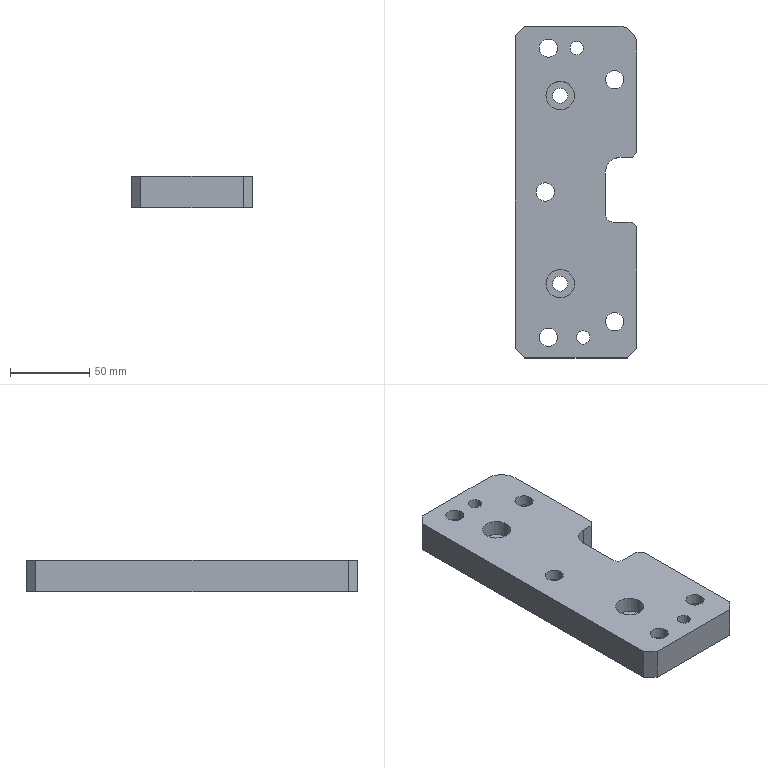Part | STEP file | lll_id3610_x_t | 1 solid | 41 faces | box 77 x 210 x 20 mm | volume 276670 mm3 | plane 22 | cylinder 19 | commonest cylinder face diameters 11.509 x5 18.007 x5 8.505 x2 9.55 x2 18 x2 10 x1
STEP:
#1=CARTESIAN_POINT('',(3739.,91.5,2.5));
#2=VERTEX_POINT('',#1);
#3=CARTESIAN_POINT('',(3739.,23.5,2.5));
#4=VERTEX_POINT('',#3);
#5=CARTESIAN_POINT('',(3739.,-58.5,2.5));
#6=DIRECTION('',(0.,-1.,0.));
#7=VECTOR('',#6,1.);
#8=LINE('',#5,#7);
#9=EDGE_CURVE('',#2,#4,#8,.T.);
#10=ORIENTED_EDGE('',*,*,#9,.F.);
#11=CARTESIAN_POINT('',(3739.,91.5,22.5));
#12=VERTEX_POINT('',#11);
#13=CARTESIAN_POINT('',(3739.,91.5,-81.5));
#14=DIRECTION('',(0.,0.,1.));
#15=VECTOR('',#14,1.);
#16=LINE('',#13,#15);
#17=EDGE_CURVE('',#2,#12,#16,.T.);
#18=ORIENTED_EDGE('',*,*,#17,.T.);
#19=CARTESIAN_POINT('',(3739.,23.5,22.5));
#20=VERTEX_POINT('',#19);
#21=CARTESIAN_POINT('',(3739.,-58.5,22.5));
#22=DIRECTION('',(0.,1.,0.));
#23=VECTOR('',#22,1.);
#24=LINE('',#21,#23);
#25=EDGE_CURVE('',#20,#12,#24,.T.);
#26=ORIENTED_EDGE('',*,*,#25,.F.);
#27=CARTESIAN_POINT('',(3739.,23.5,-81.5));
#28=DIRECTION('',(0.,0.,-1.));
#29=VECTOR('',#28,1.);
#30=LINE('',#27,#29);
#31=EDGE_CURVE('',#20,#4,#30,.T.);
#32=ORIENTED_EDGE('',*,*,#31,.T.);
#33=EDGE_LOOP('',(#10,#18,#26,#32));
#34=FACE_OUTER_BOUND('',#33,.T.);
#35=CARTESIAN_POINT('',(3739.,-58.5,-81.5));
#36=DIRECTION('',(1.,0.,0.));
#37=DIRECTION('',(0.,0.,-1.));
#38=AXIS2_PLACEMENT_3D('',#35,#36,#37);
#39=PLANE('',#38);
#40=ADVANCED_FACE('',(#34),#39,.T.);
#41=CARTESIAN_POINT('',(3690.004,-1.5,2.5));
#42=VERTEX_POINT('',#41);
#43=CARTESIAN_POINT('',(3681.,-1.5,2.5));
#44=DIRECTION('',(0.,0.,1.));
#45=DIRECTION('',(1.,0.,0.));
#46=AXIS2_PLACEMENT_3D('',#43,#44,#45);
#47=CIRCLE('',#46,9.004);
#48=EDGE_CURVE('',#42,#42,#47,.T.);
#49=ORIENTED_EDGE('',*,*,#48,.T.);
#50=EDGE_LOOP('',(#49));
#51=FACE_BOUND('',#50,.T.);
#52=CARTESIAN_POINT('',(3692.004,89.5,2.5));
#53=VERTEX_POINT('',#52);
#54=CARTESIAN_POINT('',(3683.,89.5,2.5));
#55=DIRECTION('',(0.,0.,1.));
#56=DIRECTION('',(1.,0.,0.));
#57=AXIS2_PLACEMENT_3D('',#54,#55,#56);
#58=CIRCLE('',#57,9.004);
#59=EDGE_CURVE('',#53,#53,#58,.T.);
#60=ORIENTED_EDGE('',*,*,#59,.T.);
#61=EDGE_LOOP('',(#60));
#62=FACE_BOUND('',#61,.T.);
#63=CARTESIAN_POINT('',(3705.253,89.5,2.5));
#64=VERTEX_POINT('',#63);
#65=CARTESIAN_POINT('',(3701.,89.5,2.5));
#66=DIRECTION('',(0.,0.,-1.));
#67=DIRECTION('',(1.,0.,0.));
#68=AXIS2_PLACEMENT_3D('',#65,#66,#67);
#69=CIRCLE('',#68,4.253);
#70=EDGE_CURVE('',#64,#64,#69,.T.);
#71=ORIENTED_EDGE('',*,*,#70,.F.);
#72=EDGE_LOOP('',(#71));
#73=FACE_BOUND('',#72,.T.);
#74=CARTESIAN_POINT('',(3692.004,-93.5,2.5));
#75=VERTEX_POINT('',#74);
#76=CARTESIAN_POINT('',(3683.,-93.5,2.5));
#77=DIRECTION('',(0.,0.,1.));
#78=DIRECTION('',(1.,0.,0.));
#79=AXIS2_PLACEMENT_3D('',#76,#77,#78);
#80=CIRCLE('',#79,9.004);
#81=EDGE_CURVE('',#75,#75,#80,.T.);
#82=ORIENTED_EDGE('',*,*,#81,.T.);
#83=EDGE_LOOP('',(#82));
#84=FACE_BOUND('',#83,.T.);
#85=CARTESIAN_POINT('',(3709.253,-93.5,2.5));
#86=VERTEX_POINT('',#85);
#87=CARTESIAN_POINT('',(3705.,-93.5,2.5));
#88=DIRECTION('',(0.,0.,-1.));
#89=DIRECTION('',(1.,0.,0.));
#90=AXIS2_PLACEMENT_3D('',#87,#88,#89);
#91=CIRCLE('',#90,4.253);
#92=EDGE_CURVE('',#86,#86,#91,.T.);
#93=ORIENTED_EDGE('',*,*,#92,.F.);
#94=EDGE_LOOP('',(#93));
#95=FACE_BOUND('',#94,.T.);
#96=CARTESIAN_POINT('',(3685.725,-59.5,2.5));
#97=VERTEX_POINT('',#96);
#98=CARTESIAN_POINT('',(3690.5,-59.5,2.5));
#99=DIRECTION('',(0.,0.,-1.));
#100=DIRECTION('',(-1.,0.,0.));
#101=AXIS2_PLACEMENT_3D('',#98,#99,#100);
#102=CIRCLE('',#101,4.775);
#103=EDGE_CURVE('',#97,#97,#102,.T.);
#104=ORIENTED_EDGE('',*,*,#103,.F.);
#105=EDGE_LOOP('',(#104));
#106=FACE_BOUND('',#105,.T.);
#107=CARTESIAN_POINT('',(3685.725,59.5,2.5));
#108=VERTEX_POINT('',#107);
#109=CARTESIAN_POINT('',(3690.5,59.5,2.5));
#110=DIRECTION('',(0.,0.,-1.));
#111=DIRECTION('',(-1.,0.,0.));
#112=AXIS2_PLACEMENT_3D('',#109,#110,#111);
#113=CIRCLE('',#112,4.775);
#114=EDGE_CURVE('',#108,#108,#113,.T.);
#115=ORIENTED_EDGE('',*,*,#114,.F.);
#116=EDGE_LOOP('',(#115));
#117=FACE_BOUND('',#116,.T.);
#118=CARTESIAN_POINT('',(3734.004,-83.5,2.5));
#119=VERTEX_POINT('',#118);
#120=CARTESIAN_POINT('',(3725.,-83.5,2.5));
#121=DIRECTION('',(0.,0.,1.));
#122=DIRECTION('',(1.,0.,0.));
#123=AXIS2_PLACEMENT_3D('',#120,#121,#122);
#124=CIRCLE('',#123,9.004);
#125=EDGE_CURVE('',#119,#119,#124,.T.);
#126=ORIENTED_EDGE('',*,*,#125,.T.);
#127=EDGE_LOOP('',(#126));
#128=FACE_BOUND('',#127,.T.);
#129=CARTESIAN_POINT('',(3734.004,69.5,2.5));
#130=VERTEX_POINT('',#129);
#131=CARTESIAN_POINT('',(3725.,69.5,2.5));
#132=DIRECTION('',(0.,0.,1.));
#133=DIRECTION('',(1.,0.,0.));
#134=AXIS2_PLACEMENT_3D('',#131,#132,#133);
#135=CIRCLE('',#134,9.004);
#136=EDGE_CURVE('',#130,#130,#135,.T.);
#137=ORIENTED_EDGE('',*,*,#136,.T.);
#138=EDGE_LOOP('',(#137));
#139=FACE_BOUND('',#138,.T.);
#140=CARTESIAN_POINT('',(3668.,103.5,2.5));
#141=VERTEX_POINT('',#140);
#142=CARTESIAN_POINT('',(3727.,103.5,2.5));
#143=VERTEX_POINT('',#142);
#144=CARTESIAN_POINT('',(3692.5,103.5,2.5));
#145=DIRECTION('',(1.,0.,0.));
#146=VECTOR('',#145,1.);
#147=LINE('',#144,#146);
#148=EDGE_CURVE('',#141,#143,#147,.T.);
#149=ORIENTED_EDGE('',*,*,#148,.T.);
#150=CARTESIAN_POINT('',(3727.,91.5,2.5));
#151=DIRECTION('',(0.,0.,-1.));
#152=DIRECTION('',(1.,0.,0.));
#153=AXIS2_PLACEMENT_3D('',#150,#151,#152);
#154=CIRCLE('',#153,12.);
#155=EDGE_CURVE('',#143,#2,#154,.T.);
#156=ORIENTED_EDGE('',*,*,#155,.T.);
#157=ORIENTED_EDGE('',*,*,#9,.T.);
#158=CARTESIAN_POINT('',(3736.,20.5,2.5));
#159=VERTEX_POINT('',#158);
#160=CARTESIAN_POINT('',(3814.88,99.38,2.5));
#161=DIRECTION('',(-0.7071,-0.7071,0.));
#162=VECTOR('',#161,1.);
#163=LINE('',#160,#162);
#164=EDGE_CURVE('',#4,#159,#163,.T.);
#165=ORIENTED_EDGE('',*,*,#164,.T.);
#166=CARTESIAN_POINT('',(3729.,20.5,2.5));
#167=VERTEX_POINT('',#166);
#168=CARTESIAN_POINT('',(4001.917,20.5,2.5));
#169=DIRECTION('',(-1.,0.,0.));
#170=VECTOR('',#169,1.);
#171=LINE('',#168,#170);
#172=EDGE_CURVE('',#159,#167,#171,.T.);
#173=ORIENTED_EDGE('',*,*,#172,.T.);
#174=CARTESIAN_POINT('',(3719.,10.5,2.5));
#175=VERTEX_POINT('',#174);
#176=CARTESIAN_POINT('',(3729.,10.5,2.5));
#177=DIRECTION('',(0.,0.,1.));
#178=DIRECTION('',(1.,0.,0.));
#179=AXIS2_PLACEMENT_3D('',#176,#177,#178);
#180=CIRCLE('',#179,10.);
#181=EDGE_CURVE('',#167,#175,#180,.T.);
#182=ORIENTED_EDGE('',*,*,#181,.T.);
#183=CARTESIAN_POINT('',(3719.,-15.5,2.5));
#184=VERTEX_POINT('',#183);
#185=CARTESIAN_POINT('',(3719.,-87.658,2.5));
#186=DIRECTION('',(0.,-1.,0.));
#187=VECTOR('',#186,1.);
#188=LINE('',#185,#187);
#189=EDGE_CURVE('',#175,#184,#188,.T.);
#190=ORIENTED_EDGE('',*,*,#189,.T.);
#191=CARTESIAN_POINT('',(3724.,-20.5,2.5));
#192=VERTEX_POINT('',#191);
#193=CARTESIAN_POINT('',(3724.,-15.5,2.5));
#194=DIRECTION('',(0.,0.,1.));
#195=DIRECTION('',(1.,0.,0.));
#196=AXIS2_PLACEMENT_3D('',#193,#194,#195);
#197=CIRCLE('',#196,5.);
#198=EDGE_CURVE('',#184,#192,#197,.T.);
#199=ORIENTED_EDGE('',*,*,#198,.T.);
#200=CARTESIAN_POINT('',(3736.,-20.5,2.5));
#201=VERTEX_POINT('',#200);
#202=CARTESIAN_POINT('',(4001.917,-20.5,2.5));
#203=DIRECTION('',(1.,0.,0.));
#204=VECTOR('',#203,1.);
#205=LINE('',#202,#204);
#206=EDGE_CURVE('',#192,#201,#205,.T.);
#207=ORIENTED_EDGE('',*,*,#206,.T.);
#208=CARTESIAN_POINT('',(3739.,-23.5,2.5));
#209=VERTEX_POINT('',#208);
#210=CARTESIAN_POINT('',(3902.537,-187.037,2.5));
#211=DIRECTION('',(0.7071,-0.7071,0.));
#212=VECTOR('',#211,1.);
#213=LINE('',#210,#212);
#214=EDGE_CURVE('',#201,#209,#213,.T.);
#215=ORIENTED_EDGE('',*,*,#214,.T.);
#216=CARTESIAN_POINT('',(3739.,-100.5,2.5));
#217=VERTEX_POINT('',#216);
#218=CARTESIAN_POINT('',(3739.,-58.5,2.5));
#219=DIRECTION('',(0.,-1.,0.));
#220=VECTOR('',#219,1.);
#221=LINE('',#218,#220);
#222=EDGE_CURVE('',#209,#217,#221,.T.);
#223=ORIENTED_EDGE('',*,*,#222,.T.);
#224=CARTESIAN_POINT('',(3733.,-106.5,2.5));
#225=VERTEX_POINT('',#224);
#226=CARTESIAN_POINT('',(3733.,-106.5,2.5));
#227=DIRECTION('',(-0.7071,-0.7071,0.));
#228=VECTOR('',#227,1.);
#229=LINE('',#226,#228);
#230=EDGE_CURVE('',#217,#225,#229,.T.);
#231=ORIENTED_EDGE('',*,*,#230,.T.);
#232=CARTESIAN_POINT('',(3668.,-106.5,2.5));
#233=VERTEX_POINT('',#232);
#234=CARTESIAN_POINT('',(3692.5,-106.5,2.5));
#235=DIRECTION('',(-1.,0.,0.));
#236=VECTOR('',#235,1.);
#237=LINE('',#234,#236);
#238=EDGE_CURVE('',#225,#233,#237,.T.);
#239=ORIENTED_EDGE('',*,*,#238,.T.);
#240=CARTESIAN_POINT('',(3662.,-100.5,2.5));
#241=VERTEX_POINT('',#240);
#242=CARTESIAN_POINT('',(3662.,-100.5,2.5));
#243=DIRECTION('',(-0.7071,0.7071,0.));
#244=VECTOR('',#243,1.);
#245=LINE('',#242,#244);
#246=EDGE_CURVE('',#233,#241,#245,.T.);
#247=ORIENTED_EDGE('',*,*,#246,.T.);
#248=CARTESIAN_POINT('',(3662.,97.5,2.5));
#249=VERTEX_POINT('',#248);
#250=CARTESIAN_POINT('',(3662.,-87.658,2.5));
#251=DIRECTION('',(0.,-1.,0.));
#252=VECTOR('',#251,1.);
#253=LINE('',#250,#252);
#254=EDGE_CURVE('',#249,#241,#253,.T.);
#255=ORIENTED_EDGE('',*,*,#254,.F.);
#256=CARTESIAN_POINT('',(3662.,97.5,2.5));
#257=DIRECTION('',(0.7071,0.7071,0.));
#258=VECTOR('',#257,1.);
#259=LINE('',#256,#258);
#260=EDGE_CURVE('',#249,#141,#259,.T.);
#261=ORIENTED_EDGE('',*,*,#260,.T.);
#262=EDGE_LOOP('',(#149,#156,#157,#165,#173,#182,#190,#199,#207,#215,#223,#231,#239,#247,#255,#261));
#263=FACE_BOUND('',#262,.T.);
#264=CARTESIAN_POINT('',(4001.917,-87.658,2.5));
#265=DIRECTION('',(0.,0.,1.));
#266=DIRECTION('',(0.,-1.,0.));
#267=AXIS2_PLACEMENT_3D('',#264,#265,#266);
#268=PLANE('',#267);
#269=ADVANCED_FACE('',(#51,#62,#73,#84,#95,#106,#117,#128,#139,#263),#268,.F.);
#270=CARTESIAN_POINT('',(3739.,-100.5,22.5));
#271=VERTEX_POINT('',#270);
#272=CARTESIAN_POINT('',(3739.,-23.5,22.5));
#273=VERTEX_POINT('',#272);
#274=CARTESIAN_POINT('',(3739.,-58.5,22.5));
#275=DIRECTION('',(0.,1.,0.));
#276=VECTOR('',#275,1.);
#277=LINE('',#274,#276);
#278=EDGE_CURVE('',#271,#273,#277,.T.);
#279=ORIENTED_EDGE('',*,*,#278,.F.);
#280=CARTESIAN_POINT('',(3739.,-100.5,-81.5));
#281=DIRECTION('',(0.,0.,-1.));
#282=VECTOR('',#281,1.);
#283=LINE('',#280,#282);
#284=EDGE_CURVE('',#271,#217,#283,.T.);
#285=ORIENTED_EDGE('',*,*,#284,.T.);
#286=ORIENTED_EDGE('',*,*,#222,.F.);
#287=CARTESIAN_POINT('',(3739.,-23.5,-81.5));
#288=DIRECTION('',(0.,0.,1.));
#289=VECTOR('',#288,1.);
#290=LINE('',#287,#289);
#291=EDGE_CURVE('',#209,#273,#290,.T.);
#292=ORIENTED_EDGE('',*,*,#291,.T.);
#293=EDGE_LOOP('',(#279,#285,#286,#292));
#294=FACE_OUTER_BOUND('',#293,.T.);
#295=CARTESIAN_POINT('',(3739.,-58.5,-81.5));
#296=DIRECTION('',(1.,0.,0.));
#297=DIRECTION('',(0.,0.,-1.));
#298=AXIS2_PLACEMENT_3D('',#295,#296,#297);
#299=PLANE('',#298);
#300=ADVANCED_FACE('',(#294),#299,.T.);
#301=ORIENTED_EDGE('',*,*,#103,.T.);
#302=EDGE_LOOP('',(#301));
#303=FACE_BOUND('',#302,.T.);
#304=CARTESIAN_POINT('',(3685.725,-59.5,12.5));
#305=VERTEX_POINT('',#304);
#306=CARTESIAN_POINT('',(3690.5,-59.5,12.5));
#307=DIRECTION('',(0.,0.,-1.));
#308=DIRECTION('',(-1.,0.,0.));
#309=AXIS2_PLACEMENT_3D('',#306,#307,#308);
#310=CIRCLE('',#309,4.775);
#311=EDGE_CURVE('',#305,#305,#310,.T.);
#312=ORIENTED_EDGE('',*,*,#311,.F.);
#313=EDGE_LOOP('',(#312));
#314=FACE_BOUND('',#313,.T.);
#315=CARTESIAN_POINT('',(3690.5,-59.5,-15.));
#316=DIRECTION('',(-0.000000008,0.,1.));
#317=DIRECTION('',(-1.,0.,-0.000000008));
#318=AXIS2_PLACEMENT_3D('',#315,#316,#317);
#319=CYLINDRICAL_SURFACE('',#318,4.775);
#320=ADVANCED_FACE('',(#303,#314),#319,.F.);
#321=CARTESIAN_POINT('',(3686.755,-1.5,22.5));
#322=VERTEX_POINT('',#321);
#323=CARTESIAN_POINT('',(3681.,-1.5,22.5));
#324=DIRECTION('',(0.,0.,1.));
#325=DIRECTION('',(1.,0.,0.));
#326=AXIS2_PLACEMENT_3D('',#323,#324,#325);
#327=CIRCLE('',#326,5.755);
#328=EDGE_CURVE('',#322,#322,#327,.T.);
#329=ORIENTED_EDGE('',*,*,#328,.F.);
#330=EDGE_LOOP('',(#329));
#331=FACE_BOUND('',#330,.T.);
#332=CARTESIAN_POINT('',(3730.755,69.5,22.5));
#333=VERTEX_POINT('',#332);
#334=CARTESIAN_POINT('',(3725.,69.5,22.5));
#335=DIRECTION('',(0.,0.,1.));
#336=DIRECTION('',(1.,0.,0.));
#337=AXIS2_PLACEMENT_3D('',#334,#335,#336);
#338=CIRCLE('',#337,5.755);
#339=EDGE_CURVE('',#333,#333,#338,.T.);
#340=ORIENTED_EDGE('',*,*,#339,.F.);
#341=EDGE_LOOP('',(#340));
#342=FACE_BOUND('',#341,.T.);
#343=CARTESIAN_POINT('',(3688.755,89.5,22.5));
#344=VERTEX_POINT('',#343);
#345=CARTESIAN_POINT('',(3683.,89.5,22.5));
#346=DIRECTION('',(0.,0.,1.));
#347=DIRECTION('',(1.,0.,0.));
#348=AXIS2_PLACEMENT_3D('',#345,#346,#347);
#349=CIRCLE('',#348,5.755);
#350=EDGE_CURVE('',#344,#344,#349,.T.);
#351=ORIENTED_EDGE('',*,*,#350,.F.);
#352=EDGE_LOOP('',(#351));
#353=FACE_BOUND('',#352,.T.);
#354=CARTESIAN_POINT('',(3705.253,89.5,22.5));
#355=VERTEX_POINT('',#354);
#356=CARTESIAN_POINT('',(3701.,89.5,22.5));
#357=DIRECTION('',(0.,0.,1.));
#358=DIRECTION('',(1.,0.,0.));
#359=AXIS2_PLACEMENT_3D('',#356,#357,#358);
#360=CIRCLE('',#359,4.253);
#361=EDGE_CURVE('',#355,#355,#360,.T.);
#362=ORIENTED_EDGE('',*,*,#361,.F.);
#363=EDGE_LOOP('',(#362));
#364=FACE_BOUND('',#363,.T.);
#365=CARTESIAN_POINT('',(3730.755,-83.5,22.5));
#366=VERTEX_POINT('',#365);
#367=CARTESIAN_POINT('',(3725.,-83.5,22.5));
#368=DIRECTION('',(0.,0.,1.));
#369=DIRECTION('',(1.,0.,0.));
#370=AXIS2_PLACEMENT_3D('',#367,#368,#369);
#371=CIRCLE('',#370,5.755);
#372=EDGE_CURVE('',#366,#366,#371,.T.);
#373=ORIENTED_EDGE('',*,*,#372,.F.);
#374=EDGE_LOOP('',(#373));
#375=FACE_BOUND('',#374,.T.);
#376=CARTESIAN_POINT('',(3688.755,-93.5,22.5));
#377=VERTEX_POINT('',#376);
#378=CARTESIAN_POINT('',(3683.,-93.5,22.5));
#379=DIRECTION('',(0.,0.,1.));
#380=DIRECTION('',(1.,0.,0.));
#381=AXIS2_PLACEMENT_3D('',#378,#379,#380);
#382=CIRCLE('',#381,5.755);
#383=EDGE_CURVE('',#377,#377,#382,.T.);
#384=ORIENTED_EDGE('',*,*,#383,.F.);
#385=EDGE_LOOP('',(#384));
#386=FACE_BOUND('',#385,.T.);
#387=CARTESIAN_POINT('',(3709.253,-93.5,22.5));
#388=VERTEX_POINT('',#387);
#389=CARTESIAN_POINT('',(3705.,-93.5,22.5));
#390=DIRECTION('',(0.,0.,1.));
#391=DIRECTION('',(1.,0.,0.));
#392=AXIS2_PLACEMENT_3D('',#389,#390,#391);
#393=CIRCLE('',#392,4.253);
#394=EDGE_CURVE('',#388,#388,#393,.T.);
#395=ORIENTED_EDGE('',*,*,#394,.F.);
#396=EDGE_LOOP('',(#395));
#397=FACE_BOUND('',#396,.T.);
#398=CARTESIAN_POINT('',(3681.5,-59.5,22.5));
#399=VERTEX_POINT('',#398);
#400=CARTESIAN_POINT('',(3690.5,-59.5,22.5));
#401=DIRECTION('',(0.,0.,1.));
#402=DIRECTION('',(-1.,0.,0.));
#403=AXIS2_PLACEMENT_3D('',#400,#401,#402);
#404=CIRCLE('',#403,9.);
#405=EDGE_CURVE('',#399,#399,#404,.T.);
#406=ORIENTED_EDGE('',*,*,#405,.F.);
#407=EDGE_LOOP('',(#406));
#408=FACE_BOUND('',#407,.T.);
#409=ORIENTED_EDGE('',*,*,#25,.T.);
#410=CARTESIAN_POINT('',(3727.,103.5,22.5));
#411=VERTEX_POINT('',#410);
#412=CARTESIAN_POINT('',(3727.,91.5,22.5));
#413=DIRECTION('',(0.,0.,1.));
#414=DIRECTION('',(1.,0.,0.));
#415=AXIS2_PLACEMENT_3D('',#412,#413,#414);
#416=CIRCLE('',#415,12.);
#417=EDGE_CURVE('',#12,#411,#416,.T.);
#418=ORIENTED_EDGE('',*,*,#417,.T.);
#419=CARTESIAN_POINT('',(3668.,103.5,22.5));
#420=VERTEX_POINT('',#419);
#421=CARTESIAN_POINT('',(3692.5,103.5,22.5));
#422=DIRECTION('',(-1.,0.,0.));
#423=VECTOR('',#422,1.);
#424=LINE('',#421,#423);
#425=EDGE_CURVE('',#411,#420,#424,.T.);
#426=ORIENTED_EDGE('',*,*,#425,.T.);
#427=CARTESIAN_POINT('',(3662.,97.5,22.5));
#428=VERTEX_POINT('',#427);
#429=CARTESIAN_POINT('',(3744.38,179.88,22.5));
#430=DIRECTION('',(-0.7071,-0.7071,0.));
#431=VECTOR('',#430,1.);
#432=LINE('',#429,#431);
#433=EDGE_CURVE('',#420,#428,#432,.T.);
#434=ORIENTED_EDGE('',*,*,#433,.T.);
#435=CARTESIAN_POINT('',(3662.,-100.5,22.5));
#436=VERTEX_POINT('',#435);
#437=CARTESIAN_POINT('',(3662.,-87.658,22.5));
#438=DIRECTION('',(0.,1.,0.));
#439=VECTOR('',#438,1.);
#440=LINE('',#437,#439);
#441=EDGE_CURVE('',#436,#428,#440,.T.);
#442=ORIENTED_EDGE('',*,*,#441,.F.);
#443=CARTESIAN_POINT('',(3668.,-106.5,22.5));
#444=VERTEX_POINT('',#443);
#445=CARTESIAN_POINT('',(3830.537,-269.037,22.5));
#446=DIRECTION('',(0.7071,-0.7071,0.));
#447=VECTOR('',#446,1.);
#448=LINE('',#445,#447);
#449=EDGE_CURVE('',#436,#444,#448,.T.);
#450=ORIENTED_EDGE('',*,*,#449,.T.);
#451=CARTESIAN_POINT('',(3733.,-106.5,22.5));
#452=VERTEX_POINT('',#451);
#453=CARTESIAN_POINT('',(3692.5,-106.5,22.5));
#454=DIRECTION('',(1.,0.,0.));
#455=VECTOR('',#454,1.);
#456=LINE('',#453,#455);
#457=EDGE_CURVE('',#444,#452,#456,.T.);
#458=ORIENTED_EDGE('',*,*,#457,.T.);
#459=CARTESIAN_POINT('',(3871.88,32.38,22.5));
#460=DIRECTION('',(0.7071,0.7071,0.));
#461=VECTOR('',#460,1.);
#462=LINE('',#459,#461);
#463=EDGE_CURVE('',#452,#271,#462,.T.);
#464=ORIENTED_EDGE('',*,*,#463,.T.);
#465=ORIENTED_EDGE('',*,*,#278,.T.);
#466=CARTESIAN_POINT('',(3736.,-20.5,22.5));
#467=VERTEX_POINT('',#466);
#468=CARTESIAN_POINT('',(3902.537,-187.037,22.5));
#469=DIRECTION('',(-0.7071,0.7071,0.));
#470=VECTOR('',#469,1.);
#471=LINE('',#468,#470);
#472=EDGE_CURVE('',#273,#467,#471,.T.);
#473=ORIENTED_EDGE('',*,*,#472,.T.);
#474=CARTESIAN_POINT('',(3724.,-20.5,22.5));
#475=VERTEX_POINT('',#474);
#476=CARTESIAN_POINT('',(4001.917,-20.5,22.5));
#477=DIRECTION('',(-1.,0.,0.));
#478=VECTOR('',#477,1.);
#479=LINE('',#476,#478);
#480=EDGE_CURVE('',#467,#475,#479,.T.);
#481=ORIENTED_EDGE('',*,*,#480,.T.);
#482=CARTESIAN_POINT('',(3719.,-15.5,22.5));
#483=VERTEX_POINT('',#482);
#484=CARTESIAN_POINT('',(3724.,-15.5,22.5));
#485=DIRECTION('',(0.,0.,-1.));
#486=DIRECTION('',(1.,0.,0.));
#487=AXIS2_PLACEMENT_3D('',#484,#485,#486);
#488=CIRCLE('',#487,5.);
#489=EDGE_CURVE('',#475,#483,#488,.T.);
#490=ORIENTED_EDGE('',*,*,#489,.T.);
#491=CARTESIAN_POINT('',(3719.,10.5,22.5));
#492=VERTEX_POINT('',#491);
#493=CARTESIAN_POINT('',(3719.,-87.658,22.5));
#494=DIRECTION('',(0.,1.,0.));
#495=VECTOR('',#494,1.);
#496=LINE('',#493,#495);
#497=EDGE_CURVE('',#483,#492,#496,.T.);
#498=ORIENTED_EDGE('',*,*,#497,.T.);
#499=CARTESIAN_POINT('',(3729.,20.5,22.5));
#500=VERTEX_POINT('',#499);
#501=CARTESIAN_POINT('',(3729.,10.5,22.5));
#502=DIRECTION('',(0.,0.,-1.));
#503=DIRECTION('',(1.,0.,0.));
#504=AXIS2_PLACEMENT_3D('',#501,#502,#503);
#505=CIRCLE('',#504,10.);
#506=EDGE_CURVE('',#492,#500,#505,.T.);
#507=ORIENTED_EDGE('',*,*,#506,.T.);
#508=CARTESIAN_POINT('',(3736.,20.5,22.5));
#509=VERTEX_POINT('',#508);
#510=CARTESIAN_POINT('',(3794.,20.5,22.5));
#511=DIRECTION('',(-1.,0.,0.));
#512=VECTOR('',#511,1.);
#513=LINE('',#510,#512);
#514=EDGE_CURVE('',#509,#500,#513,.T.);
#515=ORIENTED_EDGE('',*,*,#514,.F.);
#516=CARTESIAN_POINT('',(3814.88,99.38,22.5));
#517=DIRECTION('',(0.7071,0.7071,0.));
#518=VECTOR('',#517,1.);
#519=LINE('',#516,#518);
#520=EDGE_CURVE('',#509,#20,#519,.T.);
#521=ORIENTED_EDGE('',*,*,#520,.T.);
#522=EDGE_LOOP('',(#409,#418,#426,#434,#442,#450,#458,#464,#465,#473,#481,#490,#498,#507,#515,#521));
#523=FACE_BOUND('',#522,.T.);
#524=CARTESIAN_POINT('',(3681.5,59.5,22.5));
#525=VERTEX_POINT('',#524);
#526=CARTESIAN_POINT('',(3690.5,59.5,22.5));
#527=DIRECTION('',(0.,0.,1.));
#528=DIRECTION('',(-1.,0.,0.));
#529=AXIS2_PLACEMENT_3D('',#526,#527,#528);
#530=CIRCLE('',#529,9.);
#531=EDGE_CURVE('',#525,#525,#530,.T.);
#532=ORIENTED_EDGE('',*,*,#531,.F.);
#533=EDGE_LOOP('',(#532));
#534=FACE_BOUND('',#533,.T.);
#535=CARTESIAN_POINT('',(4001.917,-87.658,22.5));
#536=DIRECTION('',(0.,0.,1.));
#537=DIRECTION('',(0.,-1.,0.));
#538=AXIS2_PLACEMENT_3D('',#535,#536,#537);
#539=PLANE('',#538);
#540=ADVANCED_FACE('',(#331,#342,#353,#364,#375,#386,#397,#408,#523,#534),#539,.T.);
#541=ORIENTED_EDGE('',*,*,#457,.F.);
#542=CARTESIAN_POINT('',(3668.,-106.5,-81.5));
#543=DIRECTION('',(0.,0.,-1.));
#544=VECTOR('',#543,1.);
#545=LINE('',#542,#544);
#546=EDGE_CURVE('',#444,#233,#545,.T.);
#547=ORIENTED_EDGE('',*,*,#546,.T.);
#548=ORIENTED_EDGE('',*,*,#238,.F.);
#549=CARTESIAN_POINT('',(3733.,-106.5,-81.5));
#550=DIRECTION('',(0.,0.,1.));
#551=VECTOR('',#550,1.);
#552=LINE('',#549,#551);
#553=EDGE_CURVE('',#225,#452,#552,.T.);
#554=ORIENTED_EDGE('',*,*,#553,.T.);
#555=EDGE_LOOP('',(#541,#547,#548,#554));
#556=FACE_OUTER_BOUND('',#555,.T.);
#557=CARTESIAN_POINT('',(3692.5,-106.5,-81.5));
#558=DIRECTION('',(0.,-1.,0.));
#559=DIRECTION('',(0.,0.,-1.));
#560=AXIS2_PLACEMENT_3D('',#557,#558,#559);
#561=PLANE('',#560);
#562=ADVANCED_FACE('',(#556),#561,.T.);
#563=ORIENTED_EDGE('',*,*,#254,.T.);
#564=CARTESIAN_POINT('',(3662.,-100.5,13.5));
#565=DIRECTION('',(0.,0.,1.));
#566=VECTOR('',#565,1.);
#567=LINE('',#564,#566);
#568=EDGE_CURVE('',#241,#436,#567,.T.);
#569=ORIENTED_EDGE('',*,*,#568,.T.);
#570=ORIENTED_EDGE('',*,*,#441,.T.);
#571=CARTESIAN_POINT('',(3662.,97.5,13.5));
#572=DIRECTION('',(0.,0.,-1.));
#573=VECTOR('',#572,1.);
#574=LINE('',#571,#573);
#575=EDGE_CURVE('',#428,#249,#574,.T.);
#576=ORIENTED_EDGE('',*,*,#575,.T.);
#577=EDGE_LOOP('',(#563,#569,#570,#576));
#578=FACE_OUTER_BOUND('',#577,.T.);
#579=CARTESIAN_POINT('',(3662.,-58.5,13.5));
#580=DIRECTION('',(-1.,0.,0.));
#581=DIRECTION('',(0.,0.,1.));
#582=AXIS2_PLACEMENT_3D('',#579,#580,#581);
#583=PLANE('',#582);
#584=ADVANCED_FACE('',(#578),#583,.T.);
#585=CARTESIAN_POINT('',(3681.5,-59.5,12.5));
#586=VERTEX_POINT('',#585);
#587=CARTESIAN_POINT('',(3690.5,-59.5,12.5));
#588=DIRECTION('',(0.,0.,-1.));
#589=DIRECTION('',(-1.,0.,0.));
#590=AXIS2_PLACEMENT_3D('',#587,#588,#589);
#591=CIRCLE('',#590,9.);
#592=EDGE_CURVE('',#586,#586,#591,.T.);
#593=ORIENTED_EDGE('',*,*,#592,.F.);
#594=EDGE_LOOP('',(#593));
#595=FACE_BOUND('',#594,.T.);
#596=ORIENTED_EDGE('',*,*,#311,.T.);
#597=EDGE_LOOP('',(#596));
#598=FACE_BOUND('',#597,.T.);
#599=CARTESIAN_POINT('',(3690.5,-59.5,12.5));
#600=DIRECTION('',(0.,0.,1.));
#601=DIRECTION('',(-1.,0.,0.));
#602=AXIS2_PLACEMENT_3D('',#599,#600,#601);
#603=PLANE('',#602);
#604=ADVANCED_FACE('',(#595,#598),#603,.T.);
#605=ORIENTED_EDGE('',*,*,#405,.T.);
#606=EDGE_LOOP('',(#605));
#607=FACE_BOUND('',#606,.T.);
#608=ORIENTED_EDGE('',*,*,#592,.T.);
#609=EDGE_LOOP('',(#608));
#610=FACE_BOUND('',#609,.T.);
#611=CARTESIAN_POINT('',(3690.5,-59.5,14.5));
#612=DIRECTION('',(0.,0.,1.));
#613=DIRECTION('',(-1.,0.,0.));
#614=AXIS2_PLACEMENT_3D('',#611,#612,#613);
#615=CYLINDRICAL_SURFACE('',#614,9.);
#616=ADVANCED_FACE('',(#607,#610),#615,.F.);
#617=ORIENTED_EDGE('',*,*,#114,.T.);
#618=EDGE_LOOP('',(#617));
#619=FACE_BOUND('',#618,.T.);
#620=CARTESIAN_POINT('',(3685.725,59.5,12.5));
#621=VERTEX_POINT('',#620);
#622=CARTESIAN_POINT('',(3690.5,59.5,12.5));
#623=DIRECTION('',(0.,0.,-1.));
#624=DIRECTION('',(-1.,0.,0.));
#625=AXIS2_PLACEMENT_3D('',#622,#623,#624);
#626=CIRCLE('',#625,4.775);
#627=EDGE_CURVE('',#621,#621,#626,.T.);
#628=ORIENTED_EDGE('',*,*,#627,.F.);
#629=EDGE_LOOP('',(#628));
#630=FACE_BOUND('',#629,.T.);
#631=CARTESIAN_POINT('',(3690.5,59.5,-15.));
#632=DIRECTION('',(-0.000000008,0.,1.));
#633=DIRECTION('',(-1.,0.,-0.000000008));
#634=AXIS2_PLACEMENT_3D('',#631,#632,#633);
#635=CYLINDRICAL_SURFACE('',#634,4.775);
#636=ADVANCED_FACE('',(#619,#630),#635,.F.);
#637=ORIENTED_EDGE('',*,*,#425,.F.);
#638=CARTESIAN_POINT('',(3727.,103.5,-81.5));
#639=DIRECTION('',(0.,0.,-1.));
#640=VECTOR('',#639,1.);
#641=LINE('',#638,#640);
#642=EDGE_CURVE('',#411,#143,#641,.T.);
#643=ORIENTED_EDGE('',*,*,#642,.T.);
#644=ORIENTED_EDGE('',*,*,#148,.F.);
#645=CARTESIAN_POINT('',(3668.,103.5,-81.5));
#646=DIRECTION('',(0.,0.,1.));
#647=VECTOR('',#646,1.);
#648=LINE('',#645,#647);
#649=EDGE_CURVE('',#141,#420,#648,.T.);
#650=ORIENTED_EDGE('',*,*,#649,.T.);
#651=EDGE_LOOP('',(#637,#643,#644,#650));
#652=FACE_OUTER_BOUND('',#651,.T.);
#653=CARTESIAN_POINT('',(3692.5,103.5,-81.5));
#654=DIRECTION('',(0.,1.,0.));
#655=DIRECTION('',(0.,0.,1.));
#656=AXIS2_PLACEMENT_3D('',#653,#654,#655);
#657=PLANE('',#656);
#658=ADVANCED_FACE('',(#652),#657,.T.);
#659=CARTESIAN_POINT('',(3681.5,59.5,12.5));
#660=VERTEX_POINT('',#659);
#661=CARTESIAN_POINT('',(3690.5,59.5,12.5));
#662=DIRECTION('',(0.,0.,-1.));
#663=DIRECTION('',(-1.,0.,0.));
#664=AXIS2_PLACEMENT_3D('',#661,#662,#663);
#665=CIRCLE('',#664,9.);
#666=EDGE_CURVE('',#660,#660,#665,.T.);
#667=ORIENTED_EDGE('',*,*,#666,.F.);
#668=EDGE_LOOP('',(#667));
#669=FACE_BOUND('',#668,.T.);
#670=ORIENTED_EDGE('',*,*,#627,.T.);
#671=EDGE_LOOP('',(#670));
#672=FACE_BOUND('',#671,.T.);
#673=CARTESIAN_POINT('',(3690.5,59.5,12.5));
#674=DIRECTION('',(0.,0.,1.));
#675=DIRECTION('',(-1.,0.,0.));
#676=AXIS2_PLACEMENT_3D('',#673,#674,#675);
#677=PLANE('',#676);
#678=ADVANCED_FACE('',(#669,#672),#677,.T.);
#679=ORIENTED_EDGE('',*,*,#531,.T.);
#680=EDGE_LOOP('',(#679));
#681=FACE_BOUND('',#680,.T.);
#682=ORIENTED_EDGE('',*,*,#666,.T.);
#683=EDGE_LOOP('',(#682));
#684=FACE_BOUND('',#683,.T.);
#685=CARTESIAN_POINT('',(3690.5,59.5,14.5));
#686=DIRECTION('',(0.,0.,1.));
#687=DIRECTION('',(-1.,0.,0.));
#688=AXIS2_PLACEMENT_3D('',#685,#686,#687);
#689=CYLINDRICAL_SURFACE('',#688,9.);
#690=ADVANCED_FACE('',(#681,#684),#689,.F.);
#691=ORIENTED_EDGE('',*,*,#394,.T.);
#692=EDGE_LOOP('',(#691));
#693=FACE_BOUND('',#692,.T.);
#694=ORIENTED_EDGE('',*,*,#92,.T.);
#695=EDGE_LOOP('',(#694));
#696=FACE_BOUND('',#695,.T.);
#697=CARTESIAN_POINT('',(3705.,-93.5,-2.5));
#698=DIRECTION('',(0.,0.,1.));
#699=DIRECTION('',(1.,0.,0.));
#700=AXIS2_PLACEMENT_3D('',#697,#698,#699);
#701=CYLINDRICAL_SURFACE('',#700,4.253);
#702=ADVANCED_FACE('',(#693,#696),#701,.F.);
#703=ORIENTED_EDGE('',*,*,#383,.T.);
#704=EDGE_LOOP('',(#703));
#705=FACE_BOUND('',#704,.T.);
#706=CARTESIAN_POINT('',(3688.755,-93.5,15.5));
#707=VERTEX_POINT('',#706);
#708=CARTESIAN_POINT('',(3683.,-93.5,15.5));
#709=DIRECTION('',(0.,0.,1.));
#710=DIRECTION('',(1.,0.,0.));
#711=AXIS2_PLACEMENT_3D('',#708,#709,#710);
#712=CIRCLE('',#711,5.755);
#713=EDGE_CURVE('',#707,#707,#712,.T.);
#714=ORIENTED_EDGE('',*,*,#713,.F.);
#715=EDGE_LOOP('',(#714));
#716=FACE_BOUND('',#715,.T.);
#717=CARTESIAN_POINT('',(3683.,-93.5,-2.5));
#718=DIRECTION('',(0.,0.,1.));
#719=DIRECTION('',(1.,0.,0.));
#720=AXIS2_PLACEMENT_3D('',#717,#718,#719);
#721=CYLINDRICAL_SURFACE('',#720,5.755);
#722=ADVANCED_FACE('',(#705,#716),#721,.F.);
#723=ORIENTED_EDGE('',*,*,#713,.T.);
#724=EDGE_LOOP('',(#723));
#725=FACE_BOUND('',#724,.T.);
#726=CARTESIAN_POINT('',(3692.004,-93.5,15.5));
#727=VERTEX_POINT('',#726);
#728=CARTESIAN_POINT('',(3683.,-93.5,15.5));
#729=DIRECTION('',(0.,0.,1.));
#730=DIRECTION('',(1.,0.,0.));
#731=AXIS2_PLACEMENT_3D('',#728,#729,#730);
#732=CIRCLE('',#731,9.004);
#733=EDGE_CURVE('',#727,#727,#732,.T.);
#734=ORIENTED_EDGE('',*,*,#733,.F.);
#735=EDGE_LOOP('',(#734));
#736=FACE_BOUND('',#735,.T.);
#737=CARTESIAN_POINT('',(3683.,-93.5,15.5));
#738=DIRECTION('',(0.,0.,1.));
#739=DIRECTION('',(1.,0.,0.));
#740=AXIS2_PLACEMENT_3D('',#737,#738,#739);
#741=PLANE('',#740);
#742=ADVANCED_FACE('',(#725,#736),#741,.F.);
#743=ORIENTED_EDGE('',*,*,#733,.T.);
#744=EDGE_LOOP('',(#743));
#745=FACE_BOUND('',#744,.T.);
#746=ORIENTED_EDGE('',*,*,#81,.F.);
#747=EDGE_LOOP('',(#746));
#748=FACE_BOUND('',#747,.T.);
#749=CARTESIAN_POINT('',(3683.,-93.5,2.5));
#750=DIRECTION('',(0.,0.,1.));
#751=DIRECTION('',(1.,0.,0.));
#752=AXIS2_PLACEMENT_3D('',#749,#750,#751);
#753=CYLINDRICAL_SURFACE('',#752,9.004);
#754=ADVANCED_FACE('',(#745,#748),#753,.F.);
#755=ORIENTED_EDGE('',*,*,#372,.T.);
#756=EDGE_LOOP('',(#755));
#757=FACE_BOUND('',#756,.T.);
#758=CARTESIAN_POINT('',(3730.755,-83.5,15.5));
#759=VERTEX_POINT('',#758);
#760=CARTESIAN_POINT('',(3725.,-83.5,15.5));
#761=DIRECTION('',(0.,0.,1.));
#762=DIRECTION('',(1.,0.,0.));
#763=AXIS2_PLACEMENT_3D('',#760,#761,#762);
#764=CIRCLE('',#763,5.755);
#765=EDGE_CURVE('',#759,#759,#764,.T.);
#766=ORIENTED_EDGE('',*,*,#765,.F.);
#767=EDGE_LOOP('',(#766));
#768=FACE_BOUND('',#767,.T.);
#769=CARTESIAN_POINT('',(3725.,-83.5,-2.5));
#770=DIRECTION('',(0.,0.,1.));
#771=DIRECTION('',(1.,0.,0.));
#772=AXIS2_PLACEMENT_3D('',#769,#770,#771);
#773=CYLINDRICAL_SURFACE('',#772,5.755);
#774=ADVANCED_FACE('',(#757,#768),#773,.F.);
#775=ORIENTED_EDGE('',*,*,#765,.T.);
#776=EDGE_LOOP('',(#775));
#777=FACE_BOUND('',#776,.T.);
#778=CARTESIAN_POINT('',(3734.004,-83.5,15.5));
#779=VERTEX_POINT('',#778);
#780=CARTESIAN_POINT('',(3725.,-83.5,15.5));
#781=DIRECTION('',(0.,0.,1.));
#782=DIRECTION('',(1.,0.,0.));
#783=AXIS2_PLACEMENT_3D('',#780,#781,#782);
#784=CIRCLE('',#783,9.004);
#785=EDGE_CURVE('',#779,#779,#784,.T.);
#786=ORIENTED_EDGE('',*,*,#785,.F.);
#787=EDGE_LOOP('',(#786));
#788=FACE_BOUND('',#787,.T.);
#789=CARTESIAN_POINT('',(3725.,-83.5,15.5));
#790=DIRECTION('',(0.,0.,1.));
#791=DIRECTION('',(1.,0.,0.));
#792=AXIS2_PLACEMENT_3D('',#789,#790,#791);
#793=PLANE('',#792);
#794=ADVANCED_FACE('',(#777,#788),#793,.F.);
#795=ORIENTED_EDGE('',*,*,#785,.T.);
#796=EDGE_LOOP('',(#795));
#797=FACE_BOUND('',#796,.T.);
#798=ORIENTED_EDGE('',*,*,#125,.F.);
#799=EDGE_LOOP('',(#798));
#800=FACE_BOUND('',#799,.T.);
#801=CARTESIAN_POINT('',(3725.,-83.5,2.5));
#802=DIRECTION('',(0.,0.,1.));
#803=DIRECTION('',(1.,0.,0.));
#804=AXIS2_PLACEMENT_3D('',#801,#802,#803);
#805=CYLINDRICAL_SURFACE('',#804,9.004);
#806=ADVANCED_FACE('',(#797,#800),#805,.F.);
#807=ORIENTED_EDGE('',*,*,#70,.T.);
#808=EDGE_LOOP('',(#807));
#809=FACE_BOUND('',#808,.T.);
#810=ORIENTED_EDGE('',*,*,#361,.T.);
#811=EDGE_LOOP('',(#810));
#812=FACE_BOUND('',#811,.T.);
#813=CARTESIAN_POINT('',(3701.,89.5,-2.5));
#814=DIRECTION('',(0.,0.,1.));
#815=DIRECTION('',(1.,0.,0.));
#816=AXIS2_PLACEMENT_3D('',#813,#814,#815);
#817=CYLINDRICAL_SURFACE('',#816,4.253);
#818=ADVANCED_FACE('',(#809,#812),#817,.F.);
#819=ORIENTED_EDGE('',*,*,#350,.T.);
#820=EDGE_LOOP('',(#819));
#821=FACE_BOUND('',#820,.T.);
#822=CARTESIAN_POINT('',(3688.755,89.5,15.5));
#823=VERTEX_POINT('',#822);
#824=CARTESIAN_POINT('',(3683.,89.5,15.5));
#825=DIRECTION('',(0.,0.,1.));
#826=DIRECTION('',(1.,0.,0.));
#827=AXIS2_PLACEMENT_3D('',#824,#825,#826);
#828=CIRCLE('',#827,5.755);
#829=EDGE_CURVE('',#823,#823,#828,.T.);
#830=ORIENTED_EDGE('',*,*,#829,.F.);
#831=EDGE_LOOP('',(#830));
#832=FACE_BOUND('',#831,.T.);
#833=CARTESIAN_POINT('',(3683.,89.5,-2.5));
#834=DIRECTION('',(0.,0.,1.));
#835=DIRECTION('',(1.,0.,0.));
#836=AXIS2_PLACEMENT_3D('',#833,#834,#835);
#837=CYLINDRICAL_SURFACE('',#836,5.755);
#838=ADVANCED_FACE('',(#821,#832),#837,.F.);
#839=ORIENTED_EDGE('',*,*,#829,.T.);
#840=EDGE_LOOP('',(#839));
#841=FACE_BOUND('',#840,.T.);
#842=CARTESIAN_POINT('',(3692.004,89.5,15.5));
#843=VERTEX_POINT('',#842);
#844=CARTESIAN_POINT('',(3683.,89.5,15.5));
#845=DIRECTION('',(0.,0.,1.));
#846=DIRECTION('',(1.,0.,0.));
#847=AXIS2_PLACEMENT_3D('',#844,#845,#846);
#848=CIRCLE('',#847,9.004);
#849=EDGE_CURVE('',#843,#843,#848,.T.);
#850=ORIENTED_EDGE('',*,*,#849,.F.);
#851=EDGE_LOOP('',(#850));
#852=FACE_BOUND('',#851,.T.);
#853=CARTESIAN_POINT('',(3683.,89.5,15.5));
#854=DIRECTION('',(0.,0.,1.));
#855=DIRECTION('',(1.,0.,0.));
#856=AXIS2_PLACEMENT_3D('',#853,#854,#855);
#857=PLANE('',#856);
#858=ADVANCED_FACE('',(#841,#852),#857,.F.);
#859=ORIENTED_EDGE('',*,*,#849,.T.);
#860=EDGE_LOOP('',(#859));
#861=FACE_BOUND('',#860,.T.);
#862=ORIENTED_EDGE('',*,*,#59,.F.);
#863=EDGE_LOOP('',(#862));
#864=FACE_BOUND('',#863,.T.);
#865=CARTESIAN_POINT('',(3683.,89.5,2.5));
#866=DIRECTION('',(0.,0.,1.));
#867=DIRECTION('',(1.,0.,0.));
#868=AXIS2_PLACEMENT_3D('',#865,#866,#867);
#869=CYLINDRICAL_SURFACE('',#868,9.004);
#870=ADVANCED_FACE('',(#861,#864),#869,.F.);
#871=ORIENTED_EDGE('',*,*,#339,.T.);
#872=EDGE_LOOP('',(#871));
#873=FACE_BOUND('',#872,.T.);
#874=CARTESIAN_POINT('',(3730.755,69.5,15.5));
#875=VERTEX_POINT('',#874);
#876=CARTESIAN_POINT('',(3725.,69.5,15.5));
#877=DIRECTION('',(0.,0.,1.));
#878=DIRECTION('',(1.,0.,0.));
#879=AXIS2_PLACEMENT_3D('',#876,#877,#878);
#880=CIRCLE('',#879,5.755);
#881=EDGE_CURVE('',#875,#875,#880,.T.);
#882=ORIENTED_EDGE('',*,*,#881,.F.);
#883=EDGE_LOOP('',(#882));
#884=FACE_BOUND('',#883,.T.);
#885=CARTESIAN_POINT('',(3725.,69.5,-2.5));
#886=DIRECTION('',(0.,0.,1.));
#887=DIRECTION('',(1.,0.,0.));
#888=AXIS2_PLACEMENT_3D('',#885,#886,#887);
#889=CYLINDRICAL_SURFACE('',#888,5.755);
#890=ADVANCED_FACE('',(#873,#884),#889,.F.);
#891=ORIENTED_EDGE('',*,*,#881,.T.);
#892=EDGE_LOOP('',(#891));
#893=FACE_BOUND('',#892,.T.);
#894=CARTESIAN_POINT('',(3734.004,69.5,15.5));
#895=VERTEX_POINT('',#894);
#896=CARTESIAN_POINT('',(3725.,69.5,15.5));
#897=DIRECTION('',(0.,0.,1.));
#898=DIRECTION('',(1.,0.,0.));
#899=AXIS2_PLACEMENT_3D('',#896,#897,#898);
#900=CIRCLE('',#899,9.004);
#901=EDGE_CURVE('',#895,#895,#900,.T.);
#902=ORIENTED_EDGE('',*,*,#901,.F.);
#903=EDGE_LOOP('',(#902));
#904=FACE_BOUND('',#903,.T.);
#905=CARTESIAN_POINT('',(3725.,69.5,15.5));
#906=DIRECTION('',(0.,0.,1.));
#907=DIRECTION('',(1.,0.,0.));
#908=AXIS2_PLACEMENT_3D('',#905,#906,#907);
#909=PLANE('',#908);
#910=ADVANCED_FACE('',(#893,#904),#909,.F.);
#911=ORIENTED_EDGE('',*,*,#901,.T.);
#912=EDGE_LOOP('',(#911));
#913=FACE_BOUND('',#912,.T.);
#914=ORIENTED_EDGE('',*,*,#136,.F.);
#915=EDGE_LOOP('',(#914));
#916=FACE_BOUND('',#915,.T.);
#917=CARTESIAN_POINT('',(3725.,69.5,2.5));
#918=DIRECTION('',(0.,0.,1.));
#919=DIRECTION('',(1.,0.,0.));
#920=AXIS2_PLACEMENT_3D('',#917,#918,#919);
#921=CYLINDRICAL_SURFACE('',#920,9.004);
#922=ADVANCED_FACE('',(#913,#916),#921,.F.);
#923=ORIENTED_EDGE('',*,*,#328,.T.);
#924=EDGE_LOOP('',(#923));
#925=FACE_BOUND('',#924,.T.);
#926=CARTESIAN_POINT('',(3686.755,-1.5,15.5));
#927=VERTEX_POINT('',#926);
#928=CARTESIAN_POINT('',(3681.,-1.5,15.5));
#929=DIRECTION('',(0.,0.,1.));
#930=DIRECTION('',(1.,0.,0.));
#931=AXIS2_PLACEMENT_3D('',#928,#929,#930);
#932=CIRCLE('',#931,5.755);
#933=EDGE_CURVE('',#927,#927,#932,.T.);
#934=ORIENTED_EDGE('',*,*,#933,.F.);
#935=EDGE_LOOP('',(#934));
#936=FACE_BOUND('',#935,.T.);
#937=CARTESIAN_POINT('',(3681.,-1.5,-2.5));
#938=DIRECTION('',(0.,0.,1.));
#939=DIRECTION('',(1.,0.,0.));
#940=AXIS2_PLACEMENT_3D('',#937,#938,#939);
#941=CYLINDRICAL_SURFACE('',#940,5.755);
#942=ADVANCED_FACE('',(#925,#936),#941,.F.);
#943=ORIENTED_EDGE('',*,*,#933,.T.);
#944=EDGE_LOOP('',(#943));
#945=FACE_BOUND('',#944,.T.);
#946=CARTESIAN_POINT('',(3690.004,-1.5,15.5));
#947=VERTEX_POINT('',#946);
#948=CARTESIAN_POINT('',(3681.,-1.5,15.5));
#949=DIRECTION('',(0.,0.,1.));
#950=DIRECTION('',(1.,0.,0.));
#951=AXIS2_PLACEMENT_3D('',#948,#949,#950);
#952=CIRCLE('',#951,9.004);
#953=EDGE_CURVE('',#947,#947,#952,.T.);
#954=ORIENTED_EDGE('',*,*,#953,.F.);
#955=EDGE_LOOP('',(#954));
#956=FACE_BOUND('',#955,.T.);
#957=CARTESIAN_POINT('',(3681.,-1.5,15.5));
#958=DIRECTION('',(0.,0.,1.));
#959=DIRECTION('',(1.,0.,0.));
#960=AXIS2_PLACEMENT_3D('',#957,#958,#959);
#961=PLANE('',#960);
#962=ADVANCED_FACE('',(#945,#956),#961,.F.);
#963=ORIENTED_EDGE('',*,*,#953,.T.);
#964=EDGE_LOOP('',(#963));
#965=FACE_BOUND('',#964,.T.);
#966=ORIENTED_EDGE('',*,*,#48,.F.);
#967=EDGE_LOOP('',(#966));
#968=FACE_BOUND('',#967,.T.);
#969=CARTESIAN_POINT('',(3681.,-1.5,2.5));
#970=DIRECTION('',(0.,0.,1.));
#971=DIRECTION('',(1.,0.,0.));
#972=AXIS2_PLACEMENT_3D('',#969,#970,#971);
#973=CYLINDRICAL_SURFACE('',#972,9.004);
#974=ADVANCED_FACE('',(#965,#968),#973,.F.);
#975=ORIENTED_EDGE('',*,*,#172,.F.);
#976=CARTESIAN_POINT('',(3736.,20.5,12.5));
#977=DIRECTION('',(0.,0.,1.));
#978=VECTOR('',#977,1.);
#979=LINE('',#976,#978);
#980=EDGE_CURVE('',#159,#509,#979,.T.);
#981=ORIENTED_EDGE('',*,*,#980,.T.);
#982=ORIENTED_EDGE('',*,*,#514,.T.);
#983=CARTESIAN_POINT('',(3729.,20.5,12.5));
#984=DIRECTION('',(0.,0.,-1.));
#985=VECTOR('',#984,1.);
#986=LINE('',#983,#985);
#987=EDGE_CURVE('',#500,#167,#986,.T.);
#988=ORIENTED_EDGE('',*,*,#987,.T.);
#989=EDGE_LOOP('',(#975,#981,#982,#988));
#990=FACE_OUTER_BOUND('',#989,.T.);
#991=CARTESIAN_POINT('',(3794.,20.5,12.5));
#992=DIRECTION('',(0.,-1.,0.));
#993=DIRECTION('',(0.,0.,1.));
#994=AXIS2_PLACEMENT_3D('',#991,#992,#993);
#995=PLANE('',#994);
#996=ADVANCED_FACE('',(#990),#995,.T.);
#997=ORIENTED_EDGE('',*,*,#480,.F.);
#998=CARTESIAN_POINT('',(3736.,-20.5,12.5));
#999=DIRECTION('',(0.,0.,-1.));
#1000=VECTOR('',#999,1.);
#1001=LINE('',#998,#1000);
#1002=EDGE_CURVE('',#467,#201,#1001,.T.);
#1003=ORIENTED_EDGE('',*,*,#1002,.T.);
#1004=ORIENTED_EDGE('',*,*,#206,.F.);
#1005=CARTESIAN_POINT('',(3724.,-20.5,12.5));
#1006=DIRECTION('',(0.,0.,1.));
#1007=VECTOR('',#1006,1.);
#1008=LINE('',#1005,#1007);
#1009=EDGE_CURVE('',#192,#475,#1008,.T.);
#1010=ORIENTED_EDGE('',*,*,#1009,.T.);
#1011=EDGE_LOOP('',(#997,#1003,#1004,#1010));
#1012=FACE_OUTER_BOUND('',#1011,.T.);
#1013=CARTESIAN_POINT('',(3794.,-20.5,12.5));
#1014=DIRECTION('',(0.,1.,0.));
#1015=DIRECTION('',(0.,0.,1.));
#1016=AXIS2_PLACEMENT_3D('',#1013,#1014,#1015);
#1017=PLANE('',#1016);
#1018=ADVANCED_FACE('',(#1012),#1017,.T.);
#1019=ORIENTED_EDGE('',*,*,#189,.F.);
#1020=CARTESIAN_POINT('',(3719.,10.5,12.5));
#1021=DIRECTION('',(0.,0.,1.));
#1022=VECTOR('',#1021,1.);
#1023=LINE('',#1020,#1022);
#1024=EDGE_CURVE('',#175,#492,#1023,.T.);
#1025=ORIENTED_EDGE('',*,*,#1024,.T.);
#1026=ORIENTED_EDGE('',*,*,#497,.F.);
#1027=CARTESIAN_POINT('',(3719.,-15.5,12.5));
#1028=DIRECTION('',(0.,0.,-1.));
#1029=VECTOR('',#1028,1.);
#1030=LINE('',#1027,#1029);
#1031=EDGE_CURVE('',#483,#184,#1030,.T.);
#1032=ORIENTED_EDGE('',*,*,#1031,.T.);
#1033=EDGE_LOOP('',(#1019,#1025,#1026,#1032));
#1034=FACE_OUTER_BOUND('',#1033,.T.);
#1035=CARTESIAN_POINT('',(3719.,-26.737,12.5));
#1036=DIRECTION('',(1.,0.,0.));
#1037=DIRECTION('',(0.,0.,-1.));
#1038=AXIS2_PLACEMENT_3D('',#1035,#1036,#1037);
#1039=PLANE('',#1038);
#1040=ADVANCED_FACE('',(#1034),#1039,.T.);
#1041=ORIENTED_EDGE('',*,*,#506,.F.);
#1042=ORIENTED_EDGE('',*,*,#1024,.F.);
#1043=ORIENTED_EDGE('',*,*,#181,.F.);
#1044=ORIENTED_EDGE('',*,*,#987,.F.);
#1045=EDGE_LOOP('',(#1041,#1042,#1043,#1044));
#1046=FACE_OUTER_BOUND('',#1045,.T.);
#1047=CARTESIAN_POINT('',(3729.,10.5,12.5));
#1048=DIRECTION('',(0.,0.,-1.));
#1049=DIRECTION('',(1.,0.,0.));
#1050=AXIS2_PLACEMENT_3D('',#1047,#1048,#1049);
#1051=CYLINDRICAL_SURFACE('',#1050,10.);
#1052=ADVANCED_FACE('',(#1046),#1051,.F.);
#1053=ORIENTED_EDGE('',*,*,#489,.F.);
#1054=ORIENTED_EDGE('',*,*,#1009,.F.);
#1055=ORIENTED_EDGE('',*,*,#198,.F.);
#1056=ORIENTED_EDGE('',*,*,#1031,.F.);
#1057=EDGE_LOOP('',(#1053,#1054,#1055,#1056));
#1058=FACE_OUTER_BOUND('',#1057,.T.);
#1059=CARTESIAN_POINT('',(3724.,-15.5,12.5));
#1060=DIRECTION('',(0.,0.,-1.));
#1061=DIRECTION('',(1.,0.,0.));
#1062=AXIS2_PLACEMENT_3D('',#1059,#1060,#1061);
#1063=CYLINDRICAL_SURFACE('',#1062,5.);
#1064=ADVANCED_FACE('',(#1058),#1063,.F.);
#1065=ORIENTED_EDGE('',*,*,#520,.F.);
#1066=ORIENTED_EDGE('',*,*,#980,.F.);
#1067=ORIENTED_EDGE('',*,*,#164,.F.);
#1068=ORIENTED_EDGE('',*,*,#31,.F.);
#1069=EDGE_LOOP('',(#1065,#1066,#1067,#1068));
#1070=FACE_OUTER_BOUND('',#1069,.T.);
#1071=CARTESIAN_POINT('',(3739.,23.5,-81.5));
#1072=DIRECTION('',(-0.7071,0.7071,0.));
#1073=DIRECTION('',(0.,0.,-1.));
#1074=AXIS2_PLACEMENT_3D('',#1071,#1072,#1073);
#1075=PLANE('',#1074);
#1076=ADVANCED_FACE('',(#1070),#1075,.F.);
#1077=ORIENTED_EDGE('',*,*,#214,.F.);
#1078=ORIENTED_EDGE('',*,*,#1002,.F.);
#1079=ORIENTED_EDGE('',*,*,#472,.F.);
#1080=ORIENTED_EDGE('',*,*,#291,.F.);
#1081=EDGE_LOOP('',(#1077,#1078,#1079,#1080));
#1082=FACE_OUTER_BOUND('',#1081,.T.);
#1083=CARTESIAN_POINT('',(3739.,-23.5,-81.5));
#1084=DIRECTION('',(-0.7071,-0.7071,0.));
#1085=DIRECTION('',(0.,0.,1.));
#1086=AXIS2_PLACEMENT_3D('',#1083,#1084,#1085);
#1087=PLANE('',#1086);
#1088=ADVANCED_FACE('',(#1082),#1087,.F.);
#1089=ORIENTED_EDGE('',*,*,#246,.F.);
#1090=ORIENTED_EDGE('',*,*,#546,.F.);
#1091=ORIENTED_EDGE('',*,*,#449,.F.);
#1092=ORIENTED_EDGE('',*,*,#568,.F.);
#1093=EDGE_LOOP('',(#1089,#1090,#1091,#1092));
#1094=FACE_OUTER_BOUND('',#1093,.T.);
#1095=CARTESIAN_POINT('',(3662.,-100.5,13.5));
#1096=DIRECTION('',(0.7071,0.7071,0.));
#1097=DIRECTION('',(0.,0.,-1.));
#1098=AXIS2_PLACEMENT_3D('',#1095,#1096,#1097);
#1099=PLANE('',#1098);
#1100=ADVANCED_FACE('',(#1094),#1099,.F.);
#1101=ORIENTED_EDGE('',*,*,#230,.F.);
#1102=ORIENTED_EDGE('',*,*,#284,.F.);
#1103=ORIENTED_EDGE('',*,*,#463,.F.);
#1104=ORIENTED_EDGE('',*,*,#553,.F.);
#1105=EDGE_LOOP('',(#1101,#1102,#1103,#1104));
#1106=FACE_OUTER_BOUND('',#1105,.T.);
#1107=CARTESIAN_POINT('',(3733.,-106.5,-81.5));
#1108=DIRECTION('',(-0.7071,0.7071,0.));
#1109=DIRECTION('',(0.,0.,-1.));
#1110=AXIS2_PLACEMENT_3D('',#1107,#1108,#1109);
#1111=PLANE('',#1110);
#1112=ADVANCED_FACE('',(#1106),#1111,.F.);
#1113=ORIENTED_EDGE('',*,*,#433,.F.);
#1114=ORIENTED_EDGE('',*,*,#649,.F.);
#1115=ORIENTED_EDGE('',*,*,#260,.F.);
#1116=ORIENTED_EDGE('',*,*,#575,.F.);
#1117=EDGE_LOOP('',(#1113,#1114,#1115,#1116));
#1118=FACE_OUTER_BOUND('',#1117,.T.);
#1119=CARTESIAN_POINT('',(3662.,97.5,13.5));
#1120=DIRECTION('',(0.7071,-0.7071,0.));
#1121=DIRECTION('',(0.,0.,1.));
#1122=AXIS2_PLACEMENT_3D('',#1119,#1120,#1121);
#1123=PLANE('',#1122);
#1124=ADVANCED_FACE('',(#1118),#1123,.F.);
#1125=ORIENTED_EDGE('',*,*,#155,.F.);
#1126=ORIENTED_EDGE('',*,*,#642,.F.);
#1127=ORIENTED_EDGE('',*,*,#417,.F.);
#1128=ORIENTED_EDGE('',*,*,#17,.F.);
#1129=EDGE_LOOP('',(#1125,#1126,#1127,#1128));
#1130=FACE_OUTER_BOUND('',#1129,.T.);
#1131=CARTESIAN_POINT('',(3727.,91.5,-81.5));
#1132=DIRECTION('',(0.,0.,1.));
#1133=DIRECTION('',(-1.,0.,0.));
#1134=AXIS2_PLACEMENT_3D('',#1131,#1132,#1133);
#1135=CYLINDRICAL_SURFACE('',#1134,12.);
#1136=ADVANCED_FACE('',(#1130),#1135,.T.);
#1137=CLOSED_SHELL('',(#40,#269,#300,#320,#540,#562,#584,#604,#616,#636,#658,#678,#690,#702,#722,#742,#754,#774,#794,#806,#818,#838,#858,#870,#890,#910,#922,#942,#962,#974,#996,#1018,#1040,#1052,#1064,#1076,#1088,#1100,#1112,#1124,#1136));
#1138=MANIFOLD_SOLID_BREP('',#1137);
#1139=(LENGTH_UNIT()NAMED_UNIT(*)SI_UNIT(.MILLI.,.METRE.));
#1140=UNCERTAINTY_MEASURE_WITH_UNIT(LENGTH_MEASURE(0.00002),#1139,'','');
#1141=(NAMED_UNIT(*)PLANE_ANGLE_UNIT()SI_UNIT($,.RADIAN.));
#1142=PLANE_ANGLE_MEASURE_WITH_UNIT(PLANE_ANGLE_MEASURE(0.01745),#1141);
#1143=DIMENSIONAL_EXPONENTS(0.,0.,0.,0.,0.,0.,0.);
#1144=(CONVERSION_BASED_UNIT('DEGREE',#1142)NAMED_UNIT(#1143)PLANE_ANGLE_UNIT());
#1145=(NAMED_UNIT(*)SI_UNIT($,.STERADIAN.)SOLID_ANGLE_UNIT());
#1146=(GEOMETRIC_REPRESENTATION_CONTEXT(3)GLOBAL_UNCERTAINTY_ASSIGNED_CONTEXT((#1140))GLOBAL_UNIT_ASSIGNED_CONTEXT((#1139,#1144,#1145))REPRESENTATION_CONTEXT('',''));
#1147=ADVANCED_BREP_SHAPE_REPRESENTATION('',(#1138),#1146);